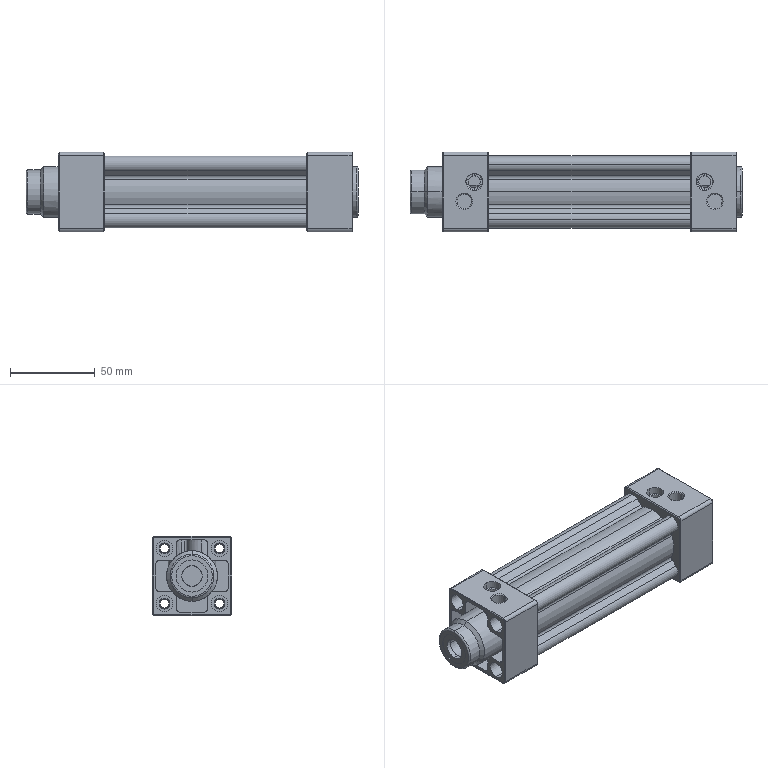Part | STEP file | 1 solid | 282 faces | box 196 x 47 x 47 mm | volume 152031 mm3 | cylinder 132 | plane 100 | cone 46 | torus 4 | commonest cylinder face diameters 4 x37 6.5 x16 9.7 x16 5.3 x8 10 x6 16 x5